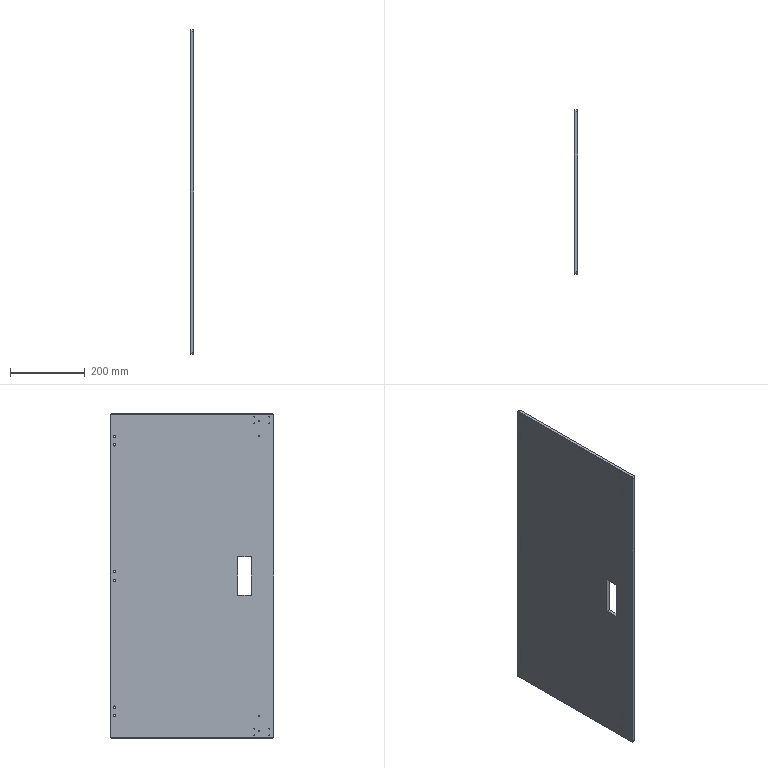Part | NX | 1 solid | 48 faces | box 10 x 438 x 869 mm | volume 3762566 mm3 | cylinder 22 | plane 18 | cone 8 | commonest cylinder face diameters 2.5 x8 6.5 x6 3.3 x4 10 x4
STEP:
#1=CARTESIAN_POINT('',(0.,-398.,-372.204));
#2=VERTEX_POINT('',#1);
#3=CARTESIAN_POINT('',(0.,-398.,-373.854));
#4=DIRECTION('',(-1.,0.,0.));
#5=DIRECTION('',(0.,0.,1.));
#6=AXIS2_PLACEMENT_3D('',#3,#4,#5);
#7=CIRCLE('',#6,1.65);
#8=EDGE_CURVE('',#2,#2,#7,.T.);
#9=ORIENTED_EDGE('',*,*,#8,.F.);
#10=EDGE_LOOP('',(#9));
#11=FACE_BOUND('',#10,.T.);
#12=CARTESIAN_POINT('',(0.,-398.,415.504));
#13=VERTEX_POINT('',#12);
#14=CARTESIAN_POINT('',(0.,-398.,413.854));
#15=DIRECTION('',(-1.,0.,0.));
#16=DIRECTION('',(0.,0.,1.));
#17=AXIS2_PLACEMENT_3D('',#14,#15,#16);
#18=CIRCLE('',#17,1.65);
#19=EDGE_CURVE('',#13,#13,#18,.T.);
#20=ORIENTED_EDGE('',*,*,#19,.F.);
#21=EDGE_LOOP('',(#20));
#22=FACE_BOUND('',#21,.T.);
#23=CARTESIAN_POINT('',(0.,-398.,375.504));
#24=VERTEX_POINT('',#23);
#25=CARTESIAN_POINT('',(0.,-398.,373.854));
#26=DIRECTION('',(-1.,0.,0.));
#27=DIRECTION('',(0.,0.,1.));
#28=AXIS2_PLACEMENT_3D('',#25,#26,#27);
#29=CIRCLE('',#28,1.65);
#30=EDGE_CURVE('',#24,#24,#29,.T.);
#31=ORIENTED_EDGE('',*,*,#30,.F.);
#32=EDGE_LOOP('',(#31));
#33=FACE_BOUND('',#32,.T.);
#34=CARTESIAN_POINT('',(0.,-386.,407.25));
#35=VERTEX_POINT('',#34);
#36=CARTESIAN_POINT('',(0.,-386.,408.5));
#37=DIRECTION('',(1.,0.,0.));
#38=DIRECTION('',(0.,0.,-1.));
#39=AXIS2_PLACEMENT_3D('',#36,#37,#38);
#40=CIRCLE('',#39,1.25);
#41=EDGE_CURVE('',#35,#35,#40,.T.);
#42=ORIENTED_EDGE('',*,*,#41,.T.);
#43=EDGE_LOOP('',(#42));
#44=FACE_BOUND('',#43,.T.);
#45=CARTESIAN_POINT('',(0.,-426.,407.25));
#46=VERTEX_POINT('',#45);
#47=CARTESIAN_POINT('',(0.,-426.,408.5));
#48=DIRECTION('',(1.,0.,0.));
#49=DIRECTION('',(0.,0.,-1.));
#50=AXIS2_PLACEMENT_3D('',#47,#48,#49);
#51=CIRCLE('',#50,1.25);
#52=EDGE_CURVE('',#46,#46,#51,.T.);
#53=ORIENTED_EDGE('',*,*,#52,.T.);
#54=EDGE_LOOP('',(#53));
#55=FACE_BOUND('',#54,.T.);
#56=CARTESIAN_POINT('',(0.,-426.,425.25));
#57=VERTEX_POINT('',#56);
#58=CARTESIAN_POINT('',(0.,-426.,426.5));
#59=DIRECTION('',(1.,0.,0.));
#60=DIRECTION('',(0.,0.,-1.));
#61=AXIS2_PLACEMENT_3D('',#58,#59,#60);
#62=CIRCLE('',#61,1.25);
#63=EDGE_CURVE('',#57,#57,#62,.T.);
#64=ORIENTED_EDGE('',*,*,#63,.T.);
#65=EDGE_LOOP('',(#64));
#66=FACE_BOUND('',#65,.T.);
#67=CARTESIAN_POINT('',(0.,-386.,425.25));
#68=VERTEX_POINT('',#67);
#69=CARTESIAN_POINT('',(0.,-386.,426.5));
#70=DIRECTION('',(1.,0.,0.));
#71=DIRECTION('',(0.,0.,-1.));
#72=AXIS2_PLACEMENT_3D('',#69,#70,#71);
#73=CIRCLE('',#72,1.25);
#74=EDGE_CURVE('',#68,#68,#73,.T.);
#75=ORIENTED_EDGE('',*,*,#74,.T.);
#76=EDGE_LOOP('',(#75));
#77=FACE_BOUND('',#76,.T.);
#78=CARTESIAN_POINT('',(0.,-386.,-427.75));
#79=VERTEX_POINT('',#78);
#80=CARTESIAN_POINT('',(0.,-386.,-426.5));
#81=DIRECTION('',(1.,0.,0.));
#82=DIRECTION('',(0.,0.,-1.));
#83=AXIS2_PLACEMENT_3D('',#80,#81,#82);
#84=CIRCLE('',#83,1.25);
#85=EDGE_CURVE('',#79,#79,#84,.T.);
#86=ORIENTED_EDGE('',*,*,#85,.T.);
#87=EDGE_LOOP('',(#86));
#88=FACE_BOUND('',#87,.T.);
#89=CARTESIAN_POINT('',(0.,-426.,-427.75));
#90=VERTEX_POINT('',#89);
#91=CARTESIAN_POINT('',(0.,-426.,-426.5));
#92=DIRECTION('',(1.,0.,0.));
#93=DIRECTION('',(0.,0.,-1.));
#94=AXIS2_PLACEMENT_3D('',#91,#92,#93);
#95=CIRCLE('',#94,1.25);
#96=EDGE_CURVE('',#90,#90,#95,.T.);
#97=ORIENTED_EDGE('',*,*,#96,.T.);
#98=EDGE_LOOP('',(#97));
#99=FACE_BOUND('',#98,.T.);
#100=CARTESIAN_POINT('',(0.,-426.,-409.75));
#101=VERTEX_POINT('',#100);
#102=CARTESIAN_POINT('',(0.,-426.,-408.5));
#103=DIRECTION('',(1.,0.,0.));
#104=DIRECTION('',(0.,0.,-1.));
#105=AXIS2_PLACEMENT_3D('',#102,#103,#104);
#106=CIRCLE('',#105,1.25);
#107=EDGE_CURVE('',#101,#101,#106,.T.);
#108=ORIENTED_EDGE('',*,*,#107,.T.);
#109=EDGE_LOOP('',(#108));
#110=FACE_BOUND('',#109,.T.);
#111=CARTESIAN_POINT('',(0.,-386.,-409.75));
#112=VERTEX_POINT('',#111);
#113=CARTESIAN_POINT('',(0.,-386.,-408.5));
#114=DIRECTION('',(1.,0.,0.));
#115=DIRECTION('',(0.,0.,-1.));
#116=AXIS2_PLACEMENT_3D('',#113,#114,#115);
#117=CIRCLE('',#116,1.25);
#118=EDGE_CURVE('',#112,#112,#117,.T.);
#119=ORIENTED_EDGE('',*,*,#118,.T.);
#120=EDGE_LOOP('',(#119));
#121=FACE_BOUND('',#120,.T.);
#122=CARTESIAN_POINT('',(0.,-5.,433.5));
#123=VERTEX_POINT('',#122);
#124=CARTESIAN_POINT('',(0.,-1.,429.5));
#125=VERTEX_POINT('',#124);
#126=CARTESIAN_POINT('',(0.,-5.,429.5));
#127=DIRECTION('',(1.,0.,0.));
#128=DIRECTION('',(0.,0.,-1.));
#129=AXIS2_PLACEMENT_3D('',#126,#127,#128);
#130=CIRCLE('',#129,4.);
#131=EDGE_CURVE('',#123,#125,#130,.F.);
#132=ORIENTED_EDGE('',*,*,#131,.T.);
#133=CARTESIAN_POINT('',(0.,-1.,-429.5));
#134=VERTEX_POINT('',#133);
#135=CARTESIAN_POINT('',(0.,-1.,434.5));
#136=DIRECTION('',(0.,0.,-1.));
#137=VECTOR('',#136,1000.);
#138=LINE('',#135,#137);
#139=EDGE_CURVE('',#125,#134,#138,.T.);
#140=ORIENTED_EDGE('',*,*,#139,.T.);
#141=CARTESIAN_POINT('',(0.,-5.,-433.5));
#142=VERTEX_POINT('',#141);
#143=CARTESIAN_POINT('',(0.,-5.,-429.5));
#144=DIRECTION('',(1.,0.,0.));
#145=DIRECTION('',(0.,0.,-1.));
#146=AXIS2_PLACEMENT_3D('',#143,#144,#145);
#147=CIRCLE('',#146,4.);
#148=EDGE_CURVE('',#134,#142,#147,.F.);
#149=ORIENTED_EDGE('',*,*,#148,.T.);
#150=CARTESIAN_POINT('',(0.,-433.,-433.5));
#151=VERTEX_POINT('',#150);
#152=CARTESIAN_POINT('',(0.,-433.,-433.5));
#153=DIRECTION('',(0.,-1.,0.));
#154=VECTOR('',#153,1000.);
#155=LINE('',#152,#154);
#156=EDGE_CURVE('',#142,#151,#155,.T.);
#157=ORIENTED_EDGE('',*,*,#156,.T.);
#158=CARTESIAN_POINT('',(0.,-437.,-429.5));
#159=VERTEX_POINT('',#158);
#160=CARTESIAN_POINT('',(0.,-433.,-429.5));
#161=DIRECTION('',(1.,0.,0.));
#162=DIRECTION('',(0.,0.,-1.));
#163=AXIS2_PLACEMENT_3D('',#160,#161,#162);
#164=CIRCLE('',#163,4.);
#165=EDGE_CURVE('',#151,#159,#164,.F.);
#166=ORIENTED_EDGE('',*,*,#165,.T.);
#167=CARTESIAN_POINT('',(0.,-437.,429.5));
#168=VERTEX_POINT('',#167);
#169=CARTESIAN_POINT('',(0.,-437.,434.5));
#170=DIRECTION('',(0.,0.,1.));
#171=VECTOR('',#170,1000.);
#172=LINE('',#169,#171);
#173=EDGE_CURVE('',#159,#168,#172,.T.);
#174=ORIENTED_EDGE('',*,*,#173,.T.);
#175=CARTESIAN_POINT('',(0.,-433.,433.5));
#176=VERTEX_POINT('',#175);
#177=CARTESIAN_POINT('',(0.,-433.,429.5));
#178=DIRECTION('',(1.,0.,0.));
#179=DIRECTION('',(0.,0.,-1.));
#180=AXIS2_PLACEMENT_3D('',#177,#178,#179);
#181=CIRCLE('',#180,4.);
#182=EDGE_CURVE('',#168,#176,#181,.F.);
#183=ORIENTED_EDGE('',*,*,#182,.T.);
#184=CARTESIAN_POINT('',(0.,-438.,433.5));
#185=DIRECTION('',(0.,1.,0.));
#186=VECTOR('',#185,1000.);
#187=LINE('',#184,#186);
#188=EDGE_CURVE('',#176,#123,#187,.T.);
#189=ORIENTED_EDGE('',*,*,#188,.T.);
#190=EDGE_LOOP('',(#132,#140,#149,#157,#166,#174,#183,#189));
#191=FACE_BOUND('',#190,.T.);
#192=CARTESIAN_POINT('',(0.,-12.,-377.25));
#193=VERTEX_POINT('',#192);
#194=CARTESIAN_POINT('',(0.,-12.,-374.));
#195=DIRECTION('',(1.,0.,0.));
#196=DIRECTION('',(0.,0.,-1.));
#197=AXIS2_PLACEMENT_3D('',#194,#195,#196);
#198=CIRCLE('',#197,3.25);
#199=EDGE_CURVE('',#193,#193,#198,.T.);
#200=ORIENTED_EDGE('',*,*,#199,.T.);
#201=EDGE_LOOP('',(#200));
#202=FACE_BOUND('',#201,.T.);
#203=CARTESIAN_POINT('',(0.,-12.,-354.25));
#204=VERTEX_POINT('',#203);
#205=CARTESIAN_POINT('',(0.,-12.,-351.));
#206=DIRECTION('',(1.,0.,0.));
#207=DIRECTION('',(0.,0.,-1.));
#208=AXIS2_PLACEMENT_3D('',#205,#206,#207);
#209=CIRCLE('',#208,3.25);
#210=EDGE_CURVE('',#204,#204,#209,.T.);
#211=ORIENTED_EDGE('',*,*,#210,.T.);
#212=EDGE_LOOP('',(#211));
#213=FACE_BOUND('',#212,.T.);
#214=CARTESIAN_POINT('',(0.,-12.,347.75));
#215=VERTEX_POINT('',#214);
#216=CARTESIAN_POINT('',(0.,-12.,351.));
#217=DIRECTION('',(1.,0.,0.));
#218=DIRECTION('',(0.,0.,-1.));
#219=AXIS2_PLACEMENT_3D('',#216,#217,#218);
#220=CIRCLE('',#219,3.25);
#221=EDGE_CURVE('',#215,#215,#220,.T.);
#222=ORIENTED_EDGE('',*,*,#221,.T.);
#223=EDGE_LOOP('',(#222));
#224=FACE_BOUND('',#223,.T.);
#225=CARTESIAN_POINT('',(0.,-12.,370.75));
#226=VERTEX_POINT('',#225);
#227=CARTESIAN_POINT('',(0.,-12.,374.));
#228=DIRECTION('',(1.,0.,0.));
#229=DIRECTION('',(0.,0.,-1.));
#230=AXIS2_PLACEMENT_3D('',#227,#228,#229);
#231=CIRCLE('',#230,3.25);
#232=EDGE_CURVE('',#226,#226,#231,.T.);
#233=ORIENTED_EDGE('',*,*,#232,.T.);
#234=EDGE_LOOP('',(#233));
#235=FACE_BOUND('',#234,.T.);
#236=CARTESIAN_POINT('',(0.,-12.,8.25));
#237=VERTEX_POINT('',#236);
#238=CARTESIAN_POINT('',(0.,-12.,11.5));
#239=DIRECTION('',(1.,0.,0.));
#240=DIRECTION('',(0.,0.,-1.));
#241=AXIS2_PLACEMENT_3D('',#238,#239,#240);
#242=CIRCLE('',#241,3.25);
#243=EDGE_CURVE('',#237,#237,#242,.T.);
#244=ORIENTED_EDGE('',*,*,#243,.T.);
#245=EDGE_LOOP('',(#244));
#246=FACE_BOUND('',#245,.T.);
#247=CARTESIAN_POINT('',(0.,-12.,-14.75));
#248=VERTEX_POINT('',#247);
#249=CARTESIAN_POINT('',(0.,-12.,-11.5));
#250=DIRECTION('',(1.,0.,0.));
#251=DIRECTION('',(0.,0.,-1.));
#252=AXIS2_PLACEMENT_3D('',#249,#250,#251);
#253=CIRCLE('',#252,3.25);
#254=EDGE_CURVE('',#248,#248,#253,.T.);
#255=ORIENTED_EDGE('',*,*,#254,.T.);
#256=EDGE_LOOP('',(#255));
#257=FACE_BOUND('',#256,.T.);
#258=CARTESIAN_POINT('',(0.,-378.,51.5));
#259=VERTEX_POINT('',#258);
#260=CARTESIAN_POINT('',(0.,-378.,-51.5));
#261=VERTEX_POINT('',#260);
#262=CARTESIAN_POINT('',(0.,-378.,51.5));
#263=DIRECTION('',(0.,0.,-1.));
#264=VECTOR('',#263,1000.);
#265=LINE('',#262,#264);
#266=EDGE_CURVE('',#259,#261,#265,.T.);
#267=ORIENTED_EDGE('',*,*,#266,.T.);
#268=CARTESIAN_POINT('',(0.,-341.,-51.5));
#269=VERTEX_POINT('',#268);
#270=CARTESIAN_POINT('',(0.,-341.,-51.5));
#271=DIRECTION('',(0.,1.,0.));
#272=VECTOR('',#271,1000.);
#273=LINE('',#270,#272);
#274=EDGE_CURVE('',#261,#269,#273,.T.);
#275=ORIENTED_EDGE('',*,*,#274,.T.);
#276=CARTESIAN_POINT('',(0.,-341.,51.5));
#277=VERTEX_POINT('',#276);
#278=CARTESIAN_POINT('',(0.,-341.,51.5));
#279=DIRECTION('',(0.,0.,1.));
#280=VECTOR('',#279,1000.);
#281=LINE('',#278,#280);
#282=EDGE_CURVE('',#269,#277,#281,.T.);
#283=ORIENTED_EDGE('',*,*,#282,.T.);
#284=CARTESIAN_POINT('',(0.,-341.,51.5));
#285=DIRECTION('',(0.,-1.,0.));
#286=VECTOR('',#285,1000.);
#287=LINE('',#284,#286);
#288=EDGE_CURVE('',#277,#259,#287,.T.);
#289=ORIENTED_EDGE('',*,*,#288,.T.);
#290=EDGE_LOOP('',(#267,#275,#283,#289));
#291=FACE_BOUND('',#290,.T.);
#292=CARTESIAN_POINT('',(0.,-398.,-412.204));
#293=VERTEX_POINT('',#292);
#294=CARTESIAN_POINT('',(0.,-398.,-413.854));
#295=DIRECTION('',(-1.,0.,0.));
#296=DIRECTION('',(0.,0.,1.));
#297=AXIS2_PLACEMENT_3D('',#294,#295,#296);
#298=CIRCLE('',#297,1.65);
#299=EDGE_CURVE('',#293,#293,#298,.T.);
#300=ORIENTED_EDGE('',*,*,#299,.F.);
#301=EDGE_LOOP('',(#300));
#302=FACE_BOUND('',#301,.T.);
#303=CARTESIAN_POINT('',(0.,-438.,434.5));
#304=DIRECTION('',(1.,0.,0.));
#305=DIRECTION('',(0.,0.,-1.));
#306=AXIS2_PLACEMENT_3D('',#303,#304,#305);
#307=PLANE('',#306);
#308=ADVANCED_FACE('',(#11,#22,#33,#44,#55,#66,#77,#88,#99,#110,#121,#191,#202,#213,#224,#235,#246,#257,#291,#302),#307,.F.);
#309=CARTESIAN_POINT('',(1.,-438.,-429.5));
#310=VERTEX_POINT('',#309);
#311=CARTESIAN_POINT('',(9.,-438.,-429.5));
#312=VERTEX_POINT('',#311);
#313=CARTESIAN_POINT('',(10.,-438.,-429.5));
#314=DIRECTION('',(1.,0.,0.));
#315=VECTOR('',#314,1000.);
#316=LINE('',#313,#315);
#317=EDGE_CURVE('',#310,#312,#316,.T.);
#318=ORIENTED_EDGE('',*,*,#317,.T.);
#319=CARTESIAN_POINT('',(9.,-438.,429.5));
#320=VERTEX_POINT('',#319);
#321=CARTESIAN_POINT('',(9.,-438.,434.5));
#322=DIRECTION('',(0.,0.,1.));
#323=VECTOR('',#322,1000.);
#324=LINE('',#321,#323);
#325=EDGE_CURVE('',#312,#320,#324,.T.);
#326=ORIENTED_EDGE('',*,*,#325,.T.);
#327=CARTESIAN_POINT('',(1.,-438.,429.5));
#328=VERTEX_POINT('',#327);
#329=CARTESIAN_POINT('',(10.,-438.,429.5));
#330=DIRECTION('',(1.,0.,0.));
#331=VECTOR('',#330,1000.);
#332=LINE('',#329,#331);
#333=EDGE_CURVE('',#320,#328,#332,.F.);
#334=ORIENTED_EDGE('',*,*,#333,.T.);
#335=CARTESIAN_POINT('',(1.,-438.,434.5));
#336=DIRECTION('',(0.,0.,-1.));
#337=VECTOR('',#336,1000.);
#338=LINE('',#335,#337);
#339=EDGE_CURVE('',#328,#310,#338,.T.);
#340=ORIENTED_EDGE('',*,*,#339,.T.);
#341=EDGE_LOOP('',(#318,#326,#334,#340));
#342=FACE_BOUND('',#341,.T.);
#343=CARTESIAN_POINT('',(10.,-438.,434.5));
#344=DIRECTION('',(0.,1.,0.));
#345=DIRECTION('',(0.,0.,1.));
#346=AXIS2_PLACEMENT_3D('',#343,#344,#345);
#347=PLANE('',#346);
#348=ADVANCED_FACE('',(#342),#347,.F.);
#349=CARTESIAN_POINT('',(10.,-398.,-412.204));
#350=VERTEX_POINT('',#349);
#351=CARTESIAN_POINT('',(10.,-398.,-413.854));
#352=DIRECTION('',(-1.,0.,0.));
#353=DIRECTION('',(0.,0.,1.));
#354=AXIS2_PLACEMENT_3D('',#351,#352,#353);
#355=CIRCLE('',#354,1.65);
#356=EDGE_CURVE('',#350,#350,#355,.T.);
#357=ORIENTED_EDGE('',*,*,#356,.T.);
#358=EDGE_LOOP('',(#357));
#359=FACE_BOUND('',#358,.T.);
#360=CARTESIAN_POINT('',(10.,-398.,-372.204));
#361=VERTEX_POINT('',#360);
#362=CARTESIAN_POINT('',(10.,-398.,-373.854));
#363=DIRECTION('',(-1.,0.,0.));
#364=DIRECTION('',(0.,0.,1.));
#365=AXIS2_PLACEMENT_3D('',#362,#363,#364);
#366=CIRCLE('',#365,1.65);
#367=EDGE_CURVE('',#361,#361,#366,.T.);
#368=ORIENTED_EDGE('',*,*,#367,.T.);
#369=EDGE_LOOP('',(#368));
#370=FACE_BOUND('',#369,.T.);
#371=CARTESIAN_POINT('',(10.,-398.,415.504));
#372=VERTEX_POINT('',#371);
#373=CARTESIAN_POINT('',(10.,-398.,413.854));
#374=DIRECTION('',(-1.,0.,0.));
#375=DIRECTION('',(0.,0.,1.));
#376=AXIS2_PLACEMENT_3D('',#373,#374,#375);
#377=CIRCLE('',#376,1.65);
#378=EDGE_CURVE('',#372,#372,#377,.T.);
#379=ORIENTED_EDGE('',*,*,#378,.T.);
#380=EDGE_LOOP('',(#379));
#381=FACE_BOUND('',#380,.T.);
#382=CARTESIAN_POINT('',(10.,-398.,375.504));
#383=VERTEX_POINT('',#382);
#384=CARTESIAN_POINT('',(10.,-398.,373.854));
#385=DIRECTION('',(-1.,0.,0.));
#386=DIRECTION('',(0.,0.,1.));
#387=AXIS2_PLACEMENT_3D('',#384,#385,#386);
#388=CIRCLE('',#387,1.65);
#389=EDGE_CURVE('',#383,#383,#388,.T.);
#390=ORIENTED_EDGE('',*,*,#389,.T.);
#391=EDGE_LOOP('',(#390));
#392=FACE_BOUND('',#391,.T.);
#393=CARTESIAN_POINT('',(10.,-386.,407.25));
#394=VERTEX_POINT('',#393);
#395=CARTESIAN_POINT('',(10.,-386.,408.5));
#396=DIRECTION('',(1.,0.,0.));
#397=DIRECTION('',(0.,0.,-1.));
#398=AXIS2_PLACEMENT_3D('',#395,#396,#397);
#399=CIRCLE('',#398,1.25);
#400=EDGE_CURVE('',#394,#394,#399,.T.);
#401=ORIENTED_EDGE('',*,*,#400,.F.);
#402=EDGE_LOOP('',(#401));
#403=FACE_BOUND('',#402,.T.);
#404=CARTESIAN_POINT('',(10.,-426.,407.25));
#405=VERTEX_POINT('',#404);
#406=CARTESIAN_POINT('',(10.,-426.,408.5));
#407=DIRECTION('',(1.,0.,0.));
#408=DIRECTION('',(0.,0.,-1.));
#409=AXIS2_PLACEMENT_3D('',#406,#407,#408);
#410=CIRCLE('',#409,1.25);
#411=EDGE_CURVE('',#405,#405,#410,.T.);
#412=ORIENTED_EDGE('',*,*,#411,.F.);
#413=EDGE_LOOP('',(#412));
#414=FACE_BOUND('',#413,.T.);
#415=CARTESIAN_POINT('',(10.,-426.,425.25));
#416=VERTEX_POINT('',#415);
#417=CARTESIAN_POINT('',(10.,-426.,426.5));
#418=DIRECTION('',(1.,0.,0.));
#419=DIRECTION('',(0.,0.,-1.));
#420=AXIS2_PLACEMENT_3D('',#417,#418,#419);
#421=CIRCLE('',#420,1.25);
#422=EDGE_CURVE('',#416,#416,#421,.T.);
#423=ORIENTED_EDGE('',*,*,#422,.F.);
#424=EDGE_LOOP('',(#423));
#425=FACE_BOUND('',#424,.T.);
#426=CARTESIAN_POINT('',(10.,-386.,425.25));
#427=VERTEX_POINT('',#426);
#428=CARTESIAN_POINT('',(10.,-386.,426.5));
#429=DIRECTION('',(1.,0.,0.));
#430=DIRECTION('',(0.,0.,-1.));
#431=AXIS2_PLACEMENT_3D('',#428,#429,#430);
#432=CIRCLE('',#431,1.25);
#433=EDGE_CURVE('',#427,#427,#432,.T.);
#434=ORIENTED_EDGE('',*,*,#433,.F.);
#435=EDGE_LOOP('',(#434));
#436=FACE_BOUND('',#435,.T.);
#437=CARTESIAN_POINT('',(10.,-386.,-427.75));
#438=VERTEX_POINT('',#437);
#439=CARTESIAN_POINT('',(10.,-386.,-426.5));
#440=DIRECTION('',(1.,0.,0.));
#441=DIRECTION('',(0.,0.,-1.));
#442=AXIS2_PLACEMENT_3D('',#439,#440,#441);
#443=CIRCLE('',#442,1.25);
#444=EDGE_CURVE('',#438,#438,#443,.T.);
#445=ORIENTED_EDGE('',*,*,#444,.F.);
#446=EDGE_LOOP('',(#445));
#447=FACE_BOUND('',#446,.T.);
#448=CARTESIAN_POINT('',(10.,-426.,-427.75));
#449=VERTEX_POINT('',#448);
#450=CARTESIAN_POINT('',(10.,-426.,-426.5));
#451=DIRECTION('',(1.,0.,0.));
#452=DIRECTION('',(0.,0.,-1.));
#453=AXIS2_PLACEMENT_3D('',#450,#451,#452);
#454=CIRCLE('',#453,1.25);
#455=EDGE_CURVE('',#449,#449,#454,.T.);
#456=ORIENTED_EDGE('',*,*,#455,.F.);
#457=EDGE_LOOP('',(#456));
#458=FACE_BOUND('',#457,.T.);
#459=CARTESIAN_POINT('',(10.,-426.,-409.75));
#460=VERTEX_POINT('',#459);
#461=CARTESIAN_POINT('',(10.,-426.,-408.5));
#462=DIRECTION('',(1.,0.,0.));
#463=DIRECTION('',(0.,0.,-1.));
#464=AXIS2_PLACEMENT_3D('',#461,#462,#463);
#465=CIRCLE('',#464,1.25);
#466=EDGE_CURVE('',#460,#460,#465,.T.);
#467=ORIENTED_EDGE('',*,*,#466,.F.);
#468=EDGE_LOOP('',(#467));
#469=FACE_BOUND('',#468,.T.);
#470=CARTESIAN_POINT('',(10.,-386.,-409.75));
#471=VERTEX_POINT('',#470);
#472=CARTESIAN_POINT('',(10.,-386.,-408.5));
#473=DIRECTION('',(1.,0.,0.));
#474=DIRECTION('',(0.,0.,-1.));
#475=AXIS2_PLACEMENT_3D('',#472,#473,#474);
#476=CIRCLE('',#475,1.25);
#477=EDGE_CURVE('',#471,#471,#476,.T.);
#478=ORIENTED_EDGE('',*,*,#477,.F.);
#479=EDGE_LOOP('',(#478));
#480=FACE_BOUND('',#479,.T.);
#481=CARTESIAN_POINT('',(10.,-5.,-433.5));
#482=VERTEX_POINT('',#481);
#483=CARTESIAN_POINT('',(10.,-1.,-429.5));
#484=VERTEX_POINT('',#483);
#485=CARTESIAN_POINT('',(10.,-5.,-429.5));
#486=DIRECTION('',(-1.,0.,0.));
#487=DIRECTION('',(0.,-1.,0.));
#488=AXIS2_PLACEMENT_3D('',#485,#486,#487);
#489=CIRCLE('',#488,4.);
#490=EDGE_CURVE('',#482,#484,#489,.F.);
#491=ORIENTED_EDGE('',*,*,#490,.T.);
#492=CARTESIAN_POINT('',(10.,-1.,429.5));
#493=VERTEX_POINT('',#492);
#494=CARTESIAN_POINT('',(10.,-1.,434.5));
#495=DIRECTION('',(0.,0.,1.));
#496=VECTOR('',#495,1000.);
#497=LINE('',#494,#496);
#498=EDGE_CURVE('',#484,#493,#497,.T.);
#499=ORIENTED_EDGE('',*,*,#498,.T.);
#500=CARTESIAN_POINT('',(10.,-5.,433.5));
#501=VERTEX_POINT('',#500);
#502=CARTESIAN_POINT('',(10.,-5.,429.5));
#503=DIRECTION('',(-1.,0.,0.));
#504=DIRECTION('',(0.,-1.,0.));
#505=AXIS2_PLACEMENT_3D('',#502,#503,#504);
#506=CIRCLE('',#505,4.);
#507=EDGE_CURVE('',#493,#501,#506,.F.);
#508=ORIENTED_EDGE('',*,*,#507,.T.);
#509=CARTESIAN_POINT('',(10.,-433.,433.5));
#510=VERTEX_POINT('',#509);
#511=CARTESIAN_POINT('',(10.,0.,433.5));
#512=DIRECTION('',(0.,-1.,0.));
#513=VECTOR('',#512,1000.);
#514=LINE('',#511,#513);
#515=EDGE_CURVE('',#501,#510,#514,.T.);
#516=ORIENTED_EDGE('',*,*,#515,.T.);
#517=CARTESIAN_POINT('',(10.,-437.,429.5));
#518=VERTEX_POINT('',#517);
#519=CARTESIAN_POINT('',(10.,-433.,429.5));
#520=DIRECTION('',(-1.,0.,0.));
#521=DIRECTION('',(0.,-1.,0.));
#522=AXIS2_PLACEMENT_3D('',#519,#520,#521);
#523=CIRCLE('',#522,4.);
#524=EDGE_CURVE('',#510,#518,#523,.F.);
#525=ORIENTED_EDGE('',*,*,#524,.T.);
#526=CARTESIAN_POINT('',(10.,-437.,-429.5));
#527=VERTEX_POINT('',#526);
#528=CARTESIAN_POINT('',(10.,-437.,434.5));
#529=DIRECTION('',(0.,0.,-1.));
#530=VECTOR('',#529,1000.);
#531=LINE('',#528,#530);
#532=EDGE_CURVE('',#518,#527,#531,.T.);
#533=ORIENTED_EDGE('',*,*,#532,.T.);
#534=CARTESIAN_POINT('',(10.,-433.,-433.5));
#535=VERTEX_POINT('',#534);
#536=CARTESIAN_POINT('',(10.,-433.,-429.5));
#537=DIRECTION('',(-1.,0.,0.));
#538=DIRECTION('',(0.,-1.,0.));
#539=AXIS2_PLACEMENT_3D('',#536,#537,#538);
#540=CIRCLE('',#539,4.);
#541=EDGE_CURVE('',#527,#535,#540,.F.);
#542=ORIENTED_EDGE('',*,*,#541,.T.);
#543=CARTESIAN_POINT('',(10.,-5.,-433.5));
#544=DIRECTION('',(0.,1.,0.));
#545=VECTOR('',#544,1000.);
#546=LINE('',#543,#545);
#547=EDGE_CURVE('',#535,#482,#546,.T.);
#548=ORIENTED_EDGE('',*,*,#547,.T.);
#549=EDGE_LOOP('',(#491,#499,#508,#516,#525,#533,#542,#548));
#550=FACE_BOUND('',#549,.T.);
#551=CARTESIAN_POINT('',(10.,-12.,-377.25));
#552=VERTEX_POINT('',#551);
#553=CARTESIAN_POINT('',(10.,-12.,-374.));
#554=DIRECTION('',(1.,0.,0.));
#555=DIRECTION('',(0.,0.,-1.));
#556=AXIS2_PLACEMENT_3D('',#553,#554,#555);
#557=CIRCLE('',#556,3.25);
#558=EDGE_CURVE('',#552,#552,#557,.T.);
#559=ORIENTED_EDGE('',*,*,#558,.F.);
#560=EDGE_LOOP('',(#559));
#561=FACE_BOUND('',#560,.T.);
#562=CARTESIAN_POINT('',(10.,-12.,-354.25));
#563=VERTEX_POINT('',#562);
#564=CARTESIAN_POINT('',(10.,-12.,-351.));
#565=DIRECTION('',(1.,0.,0.));
#566=DIRECTION('',(0.,0.,-1.));
#567=AXIS2_PLACEMENT_3D('',#564,#565,#566);
#568=CIRCLE('',#567,3.25);
#569=EDGE_CURVE('',#563,#563,#568,.T.);
#570=ORIENTED_EDGE('',*,*,#569,.F.);
#571=EDGE_LOOP('',(#570));
#572=FACE_BOUND('',#571,.T.);
#573=CARTESIAN_POINT('',(10.,-12.,347.75));
#574=VERTEX_POINT('',#573);
#575=CARTESIAN_POINT('',(10.,-12.,351.));
#576=DIRECTION('',(1.,0.,0.));
#577=DIRECTION('',(0.,0.,-1.));
#578=AXIS2_PLACEMENT_3D('',#575,#576,#577);
#579=CIRCLE('',#578,3.25);
#580=EDGE_CURVE('',#574,#574,#579,.T.);
#581=ORIENTED_EDGE('',*,*,#580,.F.);
#582=EDGE_LOOP('',(#581));
#583=FACE_BOUND('',#582,.T.);
#584=CARTESIAN_POINT('',(10.,-12.,370.75));
#585=VERTEX_POINT('',#584);
#586=CARTESIAN_POINT('',(10.,-12.,374.));
#587=DIRECTION('',(1.,0.,0.));
#588=DIRECTION('',(0.,0.,-1.));
#589=AXIS2_PLACEMENT_3D('',#586,#587,#588);
#590=CIRCLE('',#589,3.25);
#591=EDGE_CURVE('',#585,#585,#590,.T.);
#592=ORIENTED_EDGE('',*,*,#591,.F.);
#593=EDGE_LOOP('',(#592));
#594=FACE_BOUND('',#593,.T.);
#595=CARTESIAN_POINT('',(10.,-12.,8.25));
#596=VERTEX_POINT('',#595);
#597=CARTESIAN_POINT('',(10.,-12.,11.5));
#598=DIRECTION('',(1.,0.,0.));
#599=DIRECTION('',(0.,0.,-1.));
#600=AXIS2_PLACEMENT_3D('',#597,#598,#599);
#601=CIRCLE('',#600,3.25);
#602=EDGE_CURVE('',#596,#596,#601,.T.);
#603=ORIENTED_EDGE('',*,*,#602,.F.);
#604=EDGE_LOOP('',(#603));
#605=FACE_BOUND('',#604,.T.);
#606=CARTESIAN_POINT('',(10.,-12.,-14.75));
#607=VERTEX_POINT('',#606);
#608=CARTESIAN_POINT('',(10.,-12.,-11.5));
#609=DIRECTION('',(1.,0.,0.));
#610=DIRECTION('',(0.,0.,-1.));
#611=AXIS2_PLACEMENT_3D('',#608,#609,#610);
#612=CIRCLE('',#611,3.25);
#613=EDGE_CURVE('',#607,#607,#612,.T.);
#614=ORIENTED_EDGE('',*,*,#613,.F.);
#615=EDGE_LOOP('',(#614));
#616=FACE_BOUND('',#615,.T.);
#617=CARTESIAN_POINT('',(10.,-341.,-51.5));
#618=VERTEX_POINT('',#617);
#619=CARTESIAN_POINT('',(10.,-341.,51.5));
#620=VERTEX_POINT('',#619);
#621=CARTESIAN_POINT('',(10.,-341.,51.5));
#622=DIRECTION('',(0.,0.,1.));
#623=VECTOR('',#622,1000.);
#624=LINE('',#621,#623);
#625=EDGE_CURVE('',#618,#620,#624,.T.);
#626=ORIENTED_EDGE('',*,*,#625,.F.);
#627=CARTESIAN_POINT('',(10.,-378.,-51.5));
#628=VERTEX_POINT('',#627);
#629=CARTESIAN_POINT('',(10.,-341.,-51.5));
#630=DIRECTION('',(0.,1.,0.));
#631=VECTOR('',#630,1000.);
#632=LINE('',#629,#631);
#633=EDGE_CURVE('',#628,#618,#632,.T.);
#634=ORIENTED_EDGE('',*,*,#633,.F.);
#635=CARTESIAN_POINT('',(10.,-378.,51.5));
#636=VERTEX_POINT('',#635);
#637=CARTESIAN_POINT('',(10.,-378.,51.5));
#638=DIRECTION('',(0.,0.,-1.));
#639=VECTOR('',#638,1000.);
#640=LINE('',#637,#639);
#641=EDGE_CURVE('',#636,#628,#640,.T.);
#642=ORIENTED_EDGE('',*,*,#641,.F.);
#643=CARTESIAN_POINT('',(10.,-341.,51.5));
#644=DIRECTION('',(0.,-1.,0.));
#645=VECTOR('',#644,1000.);
#646=LINE('',#643,#645);
#647=EDGE_CURVE('',#620,#636,#646,.T.);
#648=ORIENTED_EDGE('',*,*,#647,.F.);
#649=EDGE_LOOP('',(#626,#634,#642,#648));
#650=FACE_BOUND('',#649,.T.);
#651=CARTESIAN_POINT('',(10.,0.,434.5));
#652=DIRECTION('',(-1.,0.,0.));
#653=DIRECTION('',(0.,-1.,0.));
#654=AXIS2_PLACEMENT_3D('',#651,#652,#653);
#655=PLANE('',#654);
#656=ADVANCED_FACE('',(#359,#370,#381,#392,#403,#414,#425,#436,#447,#458,#469,#480,#550,#561,#572,#583,#594,#605,#616,#650),#655,.F.);
#657=CARTESIAN_POINT('',(1.,0.,429.5));
#658=VERTEX_POINT('',#657);
#659=CARTESIAN_POINT('',(9.,0.,429.5));
#660=VERTEX_POINT('',#659);
#661=CARTESIAN_POINT('',(0.,0.,429.5));
#662=DIRECTION('',(-1.,0.,0.));
#663=VECTOR('',#662,1000.);
#664=LINE('',#661,#663);
#665=EDGE_CURVE('',#658,#660,#664,.F.);
#666=ORIENTED_EDGE('',*,*,#665,.T.);
#667=CARTESIAN_POINT('',(9.,0.,-429.5));
#668=VERTEX_POINT('',#667);
#669=CARTESIAN_POINT('',(9.,0.,434.5));
#670=DIRECTION('',(0.,0.,-1.));
#671=VECTOR('',#670,1000.);
#672=LINE('',#669,#671);
#673=EDGE_CURVE('',#660,#668,#672,.T.);
#674=ORIENTED_EDGE('',*,*,#673,.T.);
#675=CARTESIAN_POINT('',(1.,0.,-429.5));
#676=VERTEX_POINT('',#675);
#677=CARTESIAN_POINT('',(0.,0.,-429.5));
#678=DIRECTION('',(-1.,0.,0.));
#679=VECTOR('',#678,1000.);
#680=LINE('',#677,#679);
#681=EDGE_CURVE('',#668,#676,#680,.T.);
#682=ORIENTED_EDGE('',*,*,#681,.T.);
#683=CARTESIAN_POINT('',(1.,0.,434.5));
#684=DIRECTION('',(0.,0.,1.));
#685=VECTOR('',#684,1000.);
#686=LINE('',#683,#685);
#687=EDGE_CURVE('',#676,#658,#686,.T.);
#688=ORIENTED_EDGE('',*,*,#687,.T.);
#689=EDGE_LOOP('',(#666,#674,#682,#688));
#690=FACE_BOUND('',#689,.T.);
#691=CARTESIAN_POINT('',(0.,0.,434.5));
#692=DIRECTION('',(0.,-1.,0.));
#693=DIRECTION('',(1.,0.,0.));
#694=AXIS2_PLACEMENT_3D('',#691,#692,#693);
#695=PLANE('',#694);
#696=ADVANCED_FACE('',(#690),#695,.F.);
#697=CARTESIAN_POINT('',(1.,-433.,434.5));
#698=VERTEX_POINT('',#697);
#699=CARTESIAN_POINT('',(9.,-433.,434.5));
#700=VERTEX_POINT('',#699);
#701=CARTESIAN_POINT('',(0.,-433.,434.5));
#702=DIRECTION('',(1.,0.,0.));
#703=VECTOR('',#702,1000.);
#704=LINE('',#701,#703);
#705=EDGE_CURVE('',#698,#700,#704,.T.);
#706=ORIENTED_EDGE('',*,*,#705,.T.);
#707=CARTESIAN_POINT('',(9.,-5.,434.5));
#708=VERTEX_POINT('',#707);
#709=CARTESIAN_POINT('',(9.,0.,434.5));
#710=DIRECTION('',(0.,1.,0.));
#711=VECTOR('',#710,1000.);
#712=LINE('',#709,#711);
#713=EDGE_CURVE('',#700,#708,#712,.T.);
#714=ORIENTED_EDGE('',*,*,#713,.T.);
#715=CARTESIAN_POINT('',(1.,-5.,434.5));
#716=VERTEX_POINT('',#715);
#717=CARTESIAN_POINT('',(0.,-5.,434.5));
#718=DIRECTION('',(-1.,0.,0.));
#719=VECTOR('',#718,1000.);
#720=LINE('',#717,#719);
#721=EDGE_CURVE('',#708,#716,#720,.T.);
#722=ORIENTED_EDGE('',*,*,#721,.T.);
#723=CARTESIAN_POINT('',(1.,0.,434.5));
#724=DIRECTION('',(0.,-1.,0.));
#725=VECTOR('',#724,1000.);
#726=LINE('',#723,#725);
#727=EDGE_CURVE('',#716,#698,#726,.T.);
#728=ORIENTED_EDGE('',*,*,#727,.T.);
#729=EDGE_LOOP('',(#706,#714,#722,#728));
#730=FACE_BOUND('',#729,.T.);
#731=CARTESIAN_POINT('',(0.,0.,434.5));
#732=DIRECTION('',(0.,0.,-1.));
#733=DIRECTION('',(-1.,0.,0.));
#734=AXIS2_PLACEMENT_3D('',#731,#732,#733);
#735=PLANE('',#734);
#736=ADVANCED_FACE('',(#730),#735,.F.);
#737=CARTESIAN_POINT('',(1.,-5.,-434.5));
#738=VERTEX_POINT('',#737);
#739=CARTESIAN_POINT('',(9.,-5.,-434.5));
#740=VERTEX_POINT('',#739);
#741=CARTESIAN_POINT('',(10.,-5.,-434.5));
#742=DIRECTION('',(-1.,0.,0.));
#743=VECTOR('',#742,1000.);
#744=LINE('',#741,#743);
#745=EDGE_CURVE('',#738,#740,#744,.F.);
#746=ORIENTED_EDGE('',*,*,#745,.T.);
#747=CARTESIAN_POINT('',(9.,-433.,-434.5));
#748=VERTEX_POINT('',#747);
#749=CARTESIAN_POINT('',(9.,-433.,-434.5));
#750=DIRECTION('',(0.,-1.,0.));
#751=VECTOR('',#750,1000.);
#752=LINE('',#749,#751);
#753=EDGE_CURVE('',#740,#748,#752,.T.);
#754=ORIENTED_EDGE('',*,*,#753,.T.);
#755=CARTESIAN_POINT('',(1.,-433.,-434.5));
#756=VERTEX_POINT('',#755);
#757=CARTESIAN_POINT('',(0.,-433.,-434.5));
#758=DIRECTION('',(1.,0.,0.));
#759=VECTOR('',#758,1000.);
#760=LINE('',#757,#759);
#761=EDGE_CURVE('',#748,#756,#760,.F.);
#762=ORIENTED_EDGE('',*,*,#761,.T.);
#763=CARTESIAN_POINT('',(1.,-5.,-434.5));
#764=DIRECTION('',(0.,1.,0.));
#765=VECTOR('',#764,1000.);
#766=LINE('',#763,#765);
#767=EDGE_CURVE('',#756,#738,#766,.T.);
#768=ORIENTED_EDGE('',*,*,#767,.T.);
#769=EDGE_LOOP('',(#746,#754,#762,#768));
#770=FACE_BOUND('',#769,.T.);
#771=CARTESIAN_POINT('',(0.,0.,-434.5));
#772=DIRECTION('',(0.,0.,-1.));
#773=DIRECTION('',(-1.,0.,0.));
#774=AXIS2_PLACEMENT_3D('',#771,#772,#773);
#775=PLANE('',#774);
#776=ADVANCED_FACE('',(#770),#775,.T.);
#777=ORIENTED_EDGE('',*,*,#633,.T.);
#778=CARTESIAN_POINT('',(0.,-341.,-51.5));
#779=DIRECTION('',(1.,0.,0.));
#780=VECTOR('',#779,1000.);
#781=LINE('',#778,#780);
#782=EDGE_CURVE('',#269,#618,#781,.T.);
#783=ORIENTED_EDGE('',*,*,#782,.F.);
#784=ORIENTED_EDGE('',*,*,#274,.F.);
#785=CARTESIAN_POINT('',(0.,-378.,-51.5));
#786=DIRECTION('',(1.,0.,0.));
#787=VECTOR('',#786,1000.);
#788=LINE('',#785,#787);
#789=EDGE_CURVE('',#261,#628,#788,.T.);
#790=ORIENTED_EDGE('',*,*,#789,.T.);
#791=EDGE_LOOP('',(#777,#783,#784,#790));
#792=FACE_BOUND('',#791,.T.);
#793=CARTESIAN_POINT('',(0.,-341.,-51.5));
#794=DIRECTION('',(0.,0.,-1.));
#795=DIRECTION('',(0.,1.,0.));
#796=AXIS2_PLACEMENT_3D('',#793,#794,#795);
#797=PLANE('',#796);
#798=ADVANCED_FACE('',(#792),#797,.F.);
#799=ORIENTED_EDGE('',*,*,#641,.T.);
#800=ORIENTED_EDGE('',*,*,#789,.F.);
#801=ORIENTED_EDGE('',*,*,#266,.F.);
#802=CARTESIAN_POINT('',(0.,-378.,51.5));
#803=DIRECTION('',(1.,0.,0.));
#804=VECTOR('',#803,1000.);
#805=LINE('',#802,#804);
#806=EDGE_CURVE('',#259,#636,#805,.T.);
#807=ORIENTED_EDGE('',*,*,#806,.T.);
#808=EDGE_LOOP('',(#799,#800,#801,#807));
#809=FACE_BOUND('',#808,.T.);
#810=CARTESIAN_POINT('',(0.,-378.,51.5));
#811=DIRECTION('',(0.,-1.,0.));
#812=DIRECTION('',(1.,0.,0.));
#813=AXIS2_PLACEMENT_3D('',#810,#811,#812);
#814=PLANE('',#813);
#815=ADVANCED_FACE('',(#809),#814,.F.);
#816=ORIENTED_EDGE('',*,*,#647,.T.);
#817=ORIENTED_EDGE('',*,*,#806,.F.);
#818=ORIENTED_EDGE('',*,*,#288,.F.);
#819=CARTESIAN_POINT('',(0.,-341.,51.5));
#820=DIRECTION('',(1.,0.,0.));
#821=VECTOR('',#820,1000.);
#822=LINE('',#819,#821);
#823=EDGE_CURVE('',#277,#620,#822,.T.);
#824=ORIENTED_EDGE('',*,*,#823,.T.);
#825=EDGE_LOOP('',(#816,#817,#818,#824));
#826=FACE_BOUND('',#825,.T.);
#827=CARTESIAN_POINT('',(0.,-341.,51.5));
#828=DIRECTION('',(0.,0.,1.));
#829=DIRECTION('',(0.,-1.,0.));
#830=AXIS2_PLACEMENT_3D('',#827,#828,#829);
#831=PLANE('',#830);
#832=ADVANCED_FACE('',(#826),#831,.F.);
#833=ORIENTED_EDGE('',*,*,#625,.T.);
#834=ORIENTED_EDGE('',*,*,#823,.F.);
#835=ORIENTED_EDGE('',*,*,#282,.F.);
#836=ORIENTED_EDGE('',*,*,#782,.T.);
#837=EDGE_LOOP('',(#833,#834,#835,#836));
#838=FACE_BOUND('',#837,.T.);
#839=CARTESIAN_POINT('',(0.,-341.,51.5));
#840=DIRECTION('',(0.,1.,0.));
#841=DIRECTION('',(-1.,0.,0.));
#842=AXIS2_PLACEMENT_3D('',#839,#840,#841);
#843=PLANE('',#842);
#844=ADVANCED_FACE('',(#838),#843,.F.);
#845=ORIENTED_EDGE('',*,*,#254,.F.);
#846=EDGE_LOOP('',(#845));
#847=FACE_BOUND('',#846,.T.);
#848=ORIENTED_EDGE('',*,*,#613,.T.);
#849=EDGE_LOOP('',(#848));
#850=FACE_BOUND('',#849,.T.);
#851=CARTESIAN_POINT('',(10.,-12.,-11.5));
#852=DIRECTION('',(1.,0.,0.));
#853=DIRECTION('',(0.,0.,-1.));
#854=AXIS2_PLACEMENT_3D('',#851,#852,#853);
#855=CYLINDRICAL_SURFACE('',#854,3.25);
#856=ADVANCED_FACE('',(#847,#850),#855,.F.);
#857=ORIENTED_EDGE('',*,*,#243,.F.);
#858=EDGE_LOOP('',(#857));
#859=FACE_BOUND('',#858,.T.);
#860=ORIENTED_EDGE('',*,*,#602,.T.);
#861=EDGE_LOOP('',(#860));
#862=FACE_BOUND('',#861,.T.);
#863=CARTESIAN_POINT('',(10.,-12.,11.5));
#864=DIRECTION('',(1.,0.,0.));
#865=DIRECTION('',(0.,0.,-1.));
#866=AXIS2_PLACEMENT_3D('',#863,#864,#865);
#867=CYLINDRICAL_SURFACE('',#866,3.25);
#868=ADVANCED_FACE('',(#859,#862),#867,.F.);
#869=ORIENTED_EDGE('',*,*,#232,.F.);
#870=EDGE_LOOP('',(#869));
#871=FACE_BOUND('',#870,.T.);
#872=ORIENTED_EDGE('',*,*,#591,.T.);
#873=EDGE_LOOP('',(#872));
#874=FACE_BOUND('',#873,.T.);
#875=CARTESIAN_POINT('',(10.,-12.,374.));
#876=DIRECTION('',(1.,0.,0.));
#877=DIRECTION('',(0.,0.,-1.));
#878=AXIS2_PLACEMENT_3D('',#875,#876,#877);
#879=CYLINDRICAL_SURFACE('',#878,3.25);
#880=ADVANCED_FACE('',(#871,#874),#879,.F.);
#881=ORIENTED_EDGE('',*,*,#221,.F.);
#882=EDGE_LOOP('',(#881));
#883=FACE_BOUND('',#882,.T.);
#884=ORIENTED_EDGE('',*,*,#580,.T.);
#885=EDGE_LOOP('',(#884));
#886=FACE_BOUND('',#885,.T.);
#887=CARTESIAN_POINT('',(10.,-12.,351.));
#888=DIRECTION('',(1.,0.,0.));
#889=DIRECTION('',(0.,0.,-1.));
#890=AXIS2_PLACEMENT_3D('',#887,#888,#889);
#891=CYLINDRICAL_SURFACE('',#890,3.25);
#892=ADVANCED_FACE('',(#883,#886),#891,.F.);
#893=ORIENTED_EDGE('',*,*,#210,.F.);
#894=EDGE_LOOP('',(#893));
#895=FACE_BOUND('',#894,.T.);
#896=ORIENTED_EDGE('',*,*,#569,.T.);
#897=EDGE_LOOP('',(#896));
#898=FACE_BOUND('',#897,.T.);
#899=CARTESIAN_POINT('',(10.,-12.,-351.));
#900=DIRECTION('',(1.,0.,0.));
#901=DIRECTION('',(0.,0.,-1.));
#902=AXIS2_PLACEMENT_3D('',#899,#900,#901);
#903=CYLINDRICAL_SURFACE('',#902,3.25);
#904=ADVANCED_FACE('',(#895,#898),#903,.F.);
#905=ORIENTED_EDGE('',*,*,#199,.F.);
#906=EDGE_LOOP('',(#905));
#907=FACE_BOUND('',#906,.T.);
#908=ORIENTED_EDGE('',*,*,#558,.T.);
#909=EDGE_LOOP('',(#908));
#910=FACE_BOUND('',#909,.T.);
#911=CARTESIAN_POINT('',(10.,-12.,-374.));
#912=DIRECTION('',(1.,0.,0.));
#913=DIRECTION('',(0.,0.,-1.));
#914=AXIS2_PLACEMENT_3D('',#911,#912,#913);
#915=CYLINDRICAL_SURFACE('',#914,3.25);
#916=ADVANCED_FACE('',(#907,#910),#915,.F.);
#917=ORIENTED_EDGE('',*,*,#721,.F.);
#918=CARTESIAN_POINT('',(9.,-5.,429.5));
#919=DIRECTION('',(-1.,0.,0.));
#920=DIRECTION('',(0.,0.,1.));
#921=AXIS2_PLACEMENT_3D('',#918,#919,#920);
#922=CIRCLE('',#921,5.);
#923=EDGE_CURVE('',#708,#660,#922,.T.);
#924=ORIENTED_EDGE('',*,*,#923,.T.);
#925=ORIENTED_EDGE('',*,*,#665,.F.);
#926=CARTESIAN_POINT('',(1.,-5.,429.5));
#927=DIRECTION('',(1.,0.,0.));
#928=DIRECTION('',(0.,0.,-1.));
#929=AXIS2_PLACEMENT_3D('',#926,#927,#928);
#930=CIRCLE('',#929,5.);
#931=EDGE_CURVE('',#658,#716,#930,.T.);
#932=ORIENTED_EDGE('',*,*,#931,.T.);
#933=EDGE_LOOP('',(#917,#924,#925,#932));
#934=FACE_BOUND('',#933,.T.);
#935=CARTESIAN_POINT('',(0.,-5.,429.5));
#936=DIRECTION('',(-1.,0.,0.));
#937=DIRECTION('',(0.,-1.,0.));
#938=AXIS2_PLACEMENT_3D('',#935,#936,#937);
#939=CYLINDRICAL_SURFACE('',#938,5.);
#940=ADVANCED_FACE('',(#934),#939,.T.);
#941=ORIENTED_EDGE('',*,*,#333,.F.);
#942=CARTESIAN_POINT('',(9.,-433.,429.5));
#943=DIRECTION('',(-1.,0.,0.));
#944=DIRECTION('',(0.,0.,1.));
#945=AXIS2_PLACEMENT_3D('',#942,#943,#944);
#946=CIRCLE('',#945,5.);
#947=EDGE_CURVE('',#320,#700,#946,.T.);
#948=ORIENTED_EDGE('',*,*,#947,.T.);
#949=ORIENTED_EDGE('',*,*,#705,.F.);
#950=CARTESIAN_POINT('',(1.,-433.,429.5));
#951=DIRECTION('',(1.,0.,0.));
#952=DIRECTION('',(0.,0.,-1.));
#953=AXIS2_PLACEMENT_3D('',#950,#951,#952);
#954=CIRCLE('',#953,5.);
#955=EDGE_CURVE('',#698,#328,#954,.T.);
#956=ORIENTED_EDGE('',*,*,#955,.T.);
#957=EDGE_LOOP('',(#941,#948,#949,#956));
#958=FACE_BOUND('',#957,.T.);
#959=CARTESIAN_POINT('',(0.,-433.,429.5));
#960=DIRECTION('',(1.,0.,0.));
#961=DIRECTION('',(0.,0.,-1.));
#962=AXIS2_PLACEMENT_3D('',#959,#960,#961);
#963=CYLINDRICAL_SURFACE('',#962,5.);
#964=ADVANCED_FACE('',(#958),#963,.T.);
#965=ORIENTED_EDGE('',*,*,#681,.F.);
#966=CARTESIAN_POINT('',(9.,-5.,-429.5));
#967=DIRECTION('',(-1.,0.,0.));
#968=DIRECTION('',(0.,0.,1.));
#969=AXIS2_PLACEMENT_3D('',#966,#967,#968);
#970=CIRCLE('',#969,5.);
#971=EDGE_CURVE('',#668,#740,#970,.T.);
#972=ORIENTED_EDGE('',*,*,#971,.T.);
#973=ORIENTED_EDGE('',*,*,#745,.F.);
#974=CARTESIAN_POINT('',(1.,-5.,-429.5));
#975=DIRECTION('',(1.,0.,0.));
#976=DIRECTION('',(0.,0.,-1.));
#977=AXIS2_PLACEMENT_3D('',#974,#975,#976);
#978=CIRCLE('',#977,5.);
#979=EDGE_CURVE('',#738,#676,#978,.T.);
#980=ORIENTED_EDGE('',*,*,#979,.T.);
#981=EDGE_LOOP('',(#965,#972,#973,#980));
#982=FACE_BOUND('',#981,.T.);
#983=CARTESIAN_POINT('',(0.,-5.,-429.5));
#984=DIRECTION('',(1.,0.,0.));
#985=DIRECTION('',(0.,1.,0.));
#986=AXIS2_PLACEMENT_3D('',#983,#984,#985);
#987=CYLINDRICAL_SURFACE('',#986,5.);
#988=ADVANCED_FACE('',(#982),#987,.T.);
#989=ORIENTED_EDGE('',*,*,#761,.F.);
#990=CARTESIAN_POINT('',(9.,-433.,-429.5));
#991=DIRECTION('',(-1.,0.,0.));
#992=DIRECTION('',(0.,0.,1.));
#993=AXIS2_PLACEMENT_3D('',#990,#991,#992);
#994=CIRCLE('',#993,5.);
#995=EDGE_CURVE('',#748,#312,#994,.T.);
#996=ORIENTED_EDGE('',*,*,#995,.T.);
#997=ORIENTED_EDGE('',*,*,#317,.F.);
#998=CARTESIAN_POINT('',(1.,-433.,-429.5));
#999=DIRECTION('',(1.,0.,0.));
#1000=DIRECTION('',(0.,0.,-1.));
#1001=AXIS2_PLACEMENT_3D('',#998,#999,#1000);
#1002=CIRCLE('',#1001,5.);
#1003=EDGE_CURVE('',#310,#756,#1002,.T.);
#1004=ORIENTED_EDGE('',*,*,#1003,.T.);
#1005=EDGE_LOOP('',(#989,#996,#997,#1004));
#1006=FACE_BOUND('',#1005,.T.);
#1007=CARTESIAN_POINT('',(10.,-433.,-429.5));
#1008=DIRECTION('',(-1.,0.,0.));
#1009=DIRECTION('',(0.,0.,1.));
#1010=AXIS2_PLACEMENT_3D('',#1007,#1008,#1009);
#1011=CYLINDRICAL_SURFACE('',#1010,5.);
#1012=ADVANCED_FACE('',(#1006),#1011,.T.);
#1013=CARTESIAN_POINT('',(10.,-437.,-429.5));
#1014=DIRECTION('',(-0.7071,-0.7071,0.));
#1015=VECTOR('',#1014,1000.);
#1016=LINE('',#1013,#1015);
#1017=EDGE_CURVE('',#527,#312,#1016,.T.);
#1018=ORIENTED_EDGE('',*,*,#1017,.F.);
#1019=ORIENTED_EDGE('',*,*,#532,.F.);
#1020=CARTESIAN_POINT('',(9.,-438.,429.5));
#1021=DIRECTION('',(0.7071,0.7071,0.));
#1022=VECTOR('',#1021,1000.);
#1023=LINE('',#1020,#1022);
#1024=EDGE_CURVE('',#320,#518,#1023,.T.);
#1025=ORIENTED_EDGE('',*,*,#1024,.F.);
#1026=ORIENTED_EDGE('',*,*,#325,.F.);
#1027=EDGE_LOOP('',(#1018,#1019,#1025,#1026));
#1028=FACE_BOUND('',#1027,.T.);
#1029=CARTESIAN_POINT('',(10.,-437.,434.5));
#1030=DIRECTION('',(-0.7071,0.7071,0.));
#1031=DIRECTION('',(0.,0.,-1.));
#1032=AXIS2_PLACEMENT_3D('',#1029,#1030,#1031);
#1033=PLANE('',#1032);
#1034=ADVANCED_FACE('',(#1028),#1033,.F.);
#1035=ORIENTED_EDGE('',*,*,#1024,.T.);
#1036=ORIENTED_EDGE('',*,*,#524,.F.);
#1037=CARTESIAN_POINT('',(9.,-433.,434.5));
#1038=DIRECTION('',(0.7071,0.,-0.7071));
#1039=VECTOR('',#1038,1000.);
#1040=LINE('',#1037,#1039);
#1041=EDGE_CURVE('',#700,#510,#1040,.T.);
#1042=ORIENTED_EDGE('',*,*,#1041,.F.);
#1043=ORIENTED_EDGE('',*,*,#947,.F.);
#1044=EDGE_LOOP('',(#1035,#1036,#1042,#1043));
#1045=FACE_BOUND('',#1044,.T.);
#1046=CARTESIAN_POINT('',(10.,-433.,429.5));
#1047=DIRECTION('',(-1.,0.,0.));
#1048=DIRECTION('',(0.,0.,1.));
#1049=AXIS2_PLACEMENT_3D('',#1046,#1047,#1048);
#1050=CONICAL_SURFACE('',#1049,4.,0.7854);
#1051=ADVANCED_FACE('',(#1045),#1050,.T.);
#1052=ORIENTED_EDGE('',*,*,#1017,.T.);
#1053=ORIENTED_EDGE('',*,*,#995,.F.);
#1054=CARTESIAN_POINT('',(10.,-433.,-433.5));
#1055=DIRECTION('',(-0.7071,0.,-0.7071));
#1056=VECTOR('',#1055,1000.);
#1057=LINE('',#1054,#1056);
#1058=EDGE_CURVE('',#535,#748,#1057,.T.);
#1059=ORIENTED_EDGE('',*,*,#1058,.F.);
#1060=ORIENTED_EDGE('',*,*,#541,.F.);
#1061=EDGE_LOOP('',(#1052,#1053,#1059,#1060));
#1062=FACE_BOUND('',#1061,.T.);
#1063=CARTESIAN_POINT('',(10.,-433.,-429.5));
#1064=DIRECTION('',(-1.,0.,0.));
#1065=DIRECTION('',(0.,0.,1.));
#1066=AXIS2_PLACEMENT_3D('',#1063,#1064,#1065);
#1067=CONICAL_SURFACE('',#1066,4.,0.7854);
#1068=ADVANCED_FACE('',(#1062),#1067,.T.);
#1069=ORIENTED_EDGE('',*,*,#1041,.T.);
#1070=ORIENTED_EDGE('',*,*,#515,.F.);
#1071=CARTESIAN_POINT('',(9.,-5.,434.5));
#1072=DIRECTION('',(0.7071,0.,-0.7071));
#1073=VECTOR('',#1072,1000.);
#1074=LINE('',#1071,#1073);
#1075=EDGE_CURVE('',#708,#501,#1074,.T.);
#1076=ORIENTED_EDGE('',*,*,#1075,.F.);
#1077=ORIENTED_EDGE('',*,*,#713,.F.);
#1078=EDGE_LOOP('',(#1069,#1070,#1076,#1077));
#1079=FACE_BOUND('',#1078,.T.);
#1080=CARTESIAN_POINT('',(9.,0.,434.5));
#1081=DIRECTION('',(-0.7071,0.,-0.7071));
#1082=DIRECTION('',(0.,1.,0.));
#1083=AXIS2_PLACEMENT_3D('',#1080,#1081,#1082);
#1084=PLANE('',#1083);
#1085=ADVANCED_FACE('',(#1079),#1084,.F.);
#1086=ORIENTED_EDGE('',*,*,#1058,.T.);
#1087=ORIENTED_EDGE('',*,*,#753,.F.);
#1088=CARTESIAN_POINT('',(10.,-5.,-433.5));
#1089=DIRECTION('',(-0.7071,0.,-0.7071));
#1090=VECTOR('',#1089,1000.);
#1091=LINE('',#1088,#1090);
#1092=EDGE_CURVE('',#482,#740,#1091,.T.);
#1093=ORIENTED_EDGE('',*,*,#1092,.F.);
#1094=ORIENTED_EDGE('',*,*,#547,.F.);
#1095=EDGE_LOOP('',(#1086,#1087,#1093,#1094));
#1096=FACE_BOUND('',#1095,.T.);
#1097=CARTESIAN_POINT('',(10.,0.,-433.5));
#1098=DIRECTION('',(0.7071,0.,-0.7071));
#1099=DIRECTION('',(0.,-1.,0.));
#1100=AXIS2_PLACEMENT_3D('',#1097,#1098,#1099);
#1101=PLANE('',#1100);
#1102=ADVANCED_FACE('',(#1096),#1101,.T.);
#1103=ORIENTED_EDGE('',*,*,#1075,.T.);
#1104=ORIENTED_EDGE('',*,*,#507,.F.);
#1105=CARTESIAN_POINT('',(9.,0.,429.5));
#1106=DIRECTION('',(0.7071,-0.7071,0.));
#1107=VECTOR('',#1106,1000.);
#1108=LINE('',#1105,#1107);
#1109=EDGE_CURVE('',#660,#493,#1108,.T.);
#1110=ORIENTED_EDGE('',*,*,#1109,.F.);
#1111=ORIENTED_EDGE('',*,*,#923,.F.);
#1112=EDGE_LOOP('',(#1103,#1104,#1110,#1111));
#1113=FACE_BOUND('',#1112,.T.);
#1114=CARTESIAN_POINT('',(10.,-5.,429.5));
#1115=DIRECTION('',(-1.,0.,0.));
#1116=DIRECTION('',(0.,0.,1.));
#1117=AXIS2_PLACEMENT_3D('',#1114,#1115,#1116);
#1118=CONICAL_SURFACE('',#1117,4.,0.7854);
#1119=ADVANCED_FACE('',(#1113),#1118,.T.);
#1120=ORIENTED_EDGE('',*,*,#1092,.T.);
#1121=ORIENTED_EDGE('',*,*,#971,.F.);
#1122=CARTESIAN_POINT('',(10.,-1.,-429.5));
#1123=DIRECTION('',(-0.7071,0.7071,0.));
#1124=VECTOR('',#1123,1000.);
#1125=LINE('',#1122,#1124);
#1126=EDGE_CURVE('',#484,#668,#1125,.T.);
#1127=ORIENTED_EDGE('',*,*,#1126,.F.);
#1128=ORIENTED_EDGE('',*,*,#490,.F.);
#1129=EDGE_LOOP('',(#1120,#1121,#1127,#1128));
#1130=FACE_BOUND('',#1129,.T.);
#1131=CARTESIAN_POINT('',(10.,-5.,-429.5));
#1132=DIRECTION('',(-1.,0.,0.));
#1133=DIRECTION('',(0.,0.,1.));
#1134=AXIS2_PLACEMENT_3D('',#1131,#1132,#1133);
#1135=CONICAL_SURFACE('',#1134,4.,0.7854);
#1136=ADVANCED_FACE('',(#1130),#1135,.T.);
#1137=ORIENTED_EDGE('',*,*,#1109,.T.);
#1138=ORIENTED_EDGE('',*,*,#498,.F.);
#1139=ORIENTED_EDGE('',*,*,#1126,.T.);
#1140=ORIENTED_EDGE('',*,*,#673,.F.);
#1141=EDGE_LOOP('',(#1137,#1138,#1139,#1140));
#1142=FACE_BOUND('',#1141,.T.);
#1143=CARTESIAN_POINT('',(9.,0.,434.5));
#1144=DIRECTION('',(-0.7071,-0.7071,0.));
#1145=DIRECTION('',(0.,0.,-1.));
#1146=AXIS2_PLACEMENT_3D('',#1143,#1144,#1145);
#1147=PLANE('',#1146);
#1148=ADVANCED_FACE('',(#1142),#1147,.F.);
#1149=CARTESIAN_POINT('',(1.,-438.,-429.5));
#1150=DIRECTION('',(-0.7071,0.7071,0.));
#1151=VECTOR('',#1150,1000.);
#1152=LINE('',#1149,#1151);
#1153=EDGE_CURVE('',#310,#159,#1152,.T.);
#1154=ORIENTED_EDGE('',*,*,#1153,.F.);
#1155=ORIENTED_EDGE('',*,*,#339,.F.);
#1156=CARTESIAN_POINT('',(0.,-437.,429.5));
#1157=DIRECTION('',(0.7071,-0.7071,0.));
#1158=VECTOR('',#1157,1000.);
#1159=LINE('',#1156,#1158);
#1160=EDGE_CURVE('',#168,#328,#1159,.T.);
#1161=ORIENTED_EDGE('',*,*,#1160,.F.);
#1162=ORIENTED_EDGE('',*,*,#173,.F.);
#1163=EDGE_LOOP('',(#1154,#1155,#1161,#1162));
#1164=FACE_BOUND('',#1163,.T.);
#1165=CARTESIAN_POINT('',(1.,-438.,434.5));
#1166=DIRECTION('',(0.7071,0.7071,0.));
#1167=DIRECTION('',(0.,0.,-1.));
#1168=AXIS2_PLACEMENT_3D('',#1165,#1166,#1167);
#1169=PLANE('',#1168);
#1170=ADVANCED_FACE('',(#1164),#1169,.F.);
#1171=ORIENTED_EDGE('',*,*,#1160,.T.);
#1172=ORIENTED_EDGE('',*,*,#955,.F.);
#1173=CARTESIAN_POINT('',(0.,-433.,433.5));
#1174=DIRECTION('',(0.7071,0.,0.7071));
#1175=VECTOR('',#1174,1000.);
#1176=LINE('',#1173,#1175);
#1177=EDGE_CURVE('',#176,#698,#1176,.T.);
#1178=ORIENTED_EDGE('',*,*,#1177,.F.);
#1179=ORIENTED_EDGE('',*,*,#182,.F.);
#1180=EDGE_LOOP('',(#1171,#1172,#1178,#1179));
#1181=FACE_BOUND('',#1180,.T.);
#1182=CARTESIAN_POINT('',(0.,-433.,429.5));
#1183=DIRECTION('',(1.,0.,0.));
#1184=DIRECTION('',(0.,0.,-1.));
#1185=AXIS2_PLACEMENT_3D('',#1182,#1183,#1184);
#1186=CONICAL_SURFACE('',#1185,4.,0.7854);
#1187=ADVANCED_FACE('',(#1181),#1186,.T.);
#1188=ORIENTED_EDGE('',*,*,#1153,.T.);
#1189=ORIENTED_EDGE('',*,*,#165,.F.);
#1190=CARTESIAN_POINT('',(1.,-433.,-434.5));
#1191=DIRECTION('',(-0.7071,0.,0.7071));
#1192=VECTOR('',#1191,1000.);
#1193=LINE('',#1190,#1192);
#1194=EDGE_CURVE('',#756,#151,#1193,.T.);
#1195=ORIENTED_EDGE('',*,*,#1194,.F.);
#1196=ORIENTED_EDGE('',*,*,#1003,.F.);
#1197=EDGE_LOOP('',(#1188,#1189,#1195,#1196));
#1198=FACE_BOUND('',#1197,.T.);
#1199=CARTESIAN_POINT('',(0.,-433.,-429.5));
#1200=DIRECTION('',(1.,0.,0.));
#1201=DIRECTION('',(0.,0.,-1.));
#1202=AXIS2_PLACEMENT_3D('',#1199,#1200,#1201);
#1203=CONICAL_SURFACE('',#1202,4.,0.7854);
#1204=ADVANCED_FACE('',(#1198),#1203,.T.);
#1205=ORIENTED_EDGE('',*,*,#1177,.T.);
#1206=ORIENTED_EDGE('',*,*,#727,.F.);
#1207=CARTESIAN_POINT('',(0.,-5.,433.5));
#1208=DIRECTION('',(0.7071,0.,0.7071));
#1209=VECTOR('',#1208,1000.);
#1210=LINE('',#1207,#1209);
#1211=EDGE_CURVE('',#123,#716,#1210,.T.);
#1212=ORIENTED_EDGE('',*,*,#1211,.F.);
#1213=ORIENTED_EDGE('',*,*,#188,.F.);
#1214=EDGE_LOOP('',(#1205,#1206,#1212,#1213));
#1215=FACE_BOUND('',#1214,.T.);
#1216=CARTESIAN_POINT('',(1.,0.,434.5));
#1217=DIRECTION('',(0.7071,0.,-0.7071));
#1218=DIRECTION('',(0.,-1.,0.));
#1219=AXIS2_PLACEMENT_3D('',#1216,#1217,#1218);
#1220=PLANE('',#1219);
#1221=ADVANCED_FACE('',(#1215),#1220,.F.);
#1222=ORIENTED_EDGE('',*,*,#1194,.T.);
#1223=ORIENTED_EDGE('',*,*,#156,.F.);
#1224=CARTESIAN_POINT('',(1.,-5.,-434.5));
#1225=DIRECTION('',(-0.7071,0.,0.7071));
#1226=VECTOR('',#1225,1000.);
#1227=LINE('',#1224,#1226);
#1228=EDGE_CURVE('',#738,#142,#1227,.T.);
#1229=ORIENTED_EDGE('',*,*,#1228,.F.);
#1230=ORIENTED_EDGE('',*,*,#767,.F.);
#1231=EDGE_LOOP('',(#1222,#1223,#1229,#1230));
#1232=FACE_BOUND('',#1231,.T.);
#1233=CARTESIAN_POINT('',(0.,-438.,-433.5));
#1234=DIRECTION('',(-0.7071,0.,-0.7071));
#1235=DIRECTION('',(0.,1.,0.));
#1236=AXIS2_PLACEMENT_3D('',#1233,#1234,#1235);
#1237=PLANE('',#1236);
#1238=ADVANCED_FACE('',(#1232),#1237,.T.);
#1239=ORIENTED_EDGE('',*,*,#1211,.T.);
#1240=ORIENTED_EDGE('',*,*,#931,.F.);
#1241=CARTESIAN_POINT('',(0.,-1.,429.5));
#1242=DIRECTION('',(0.7071,0.7071,0.));
#1243=VECTOR('',#1242,1000.);
#1244=LINE('',#1241,#1243);
#1245=EDGE_CURVE('',#125,#658,#1244,.T.);
#1246=ORIENTED_EDGE('',*,*,#1245,.F.);
#1247=ORIENTED_EDGE('',*,*,#131,.F.);
#1248=EDGE_LOOP('',(#1239,#1240,#1246,#1247));
#1249=FACE_BOUND('',#1248,.T.);
#1250=CARTESIAN_POINT('',(0.,-5.,429.5));
#1251=DIRECTION('',(1.,0.,0.));
#1252=DIRECTION('',(0.,0.,-1.));
#1253=AXIS2_PLACEMENT_3D('',#1250,#1251,#1252);
#1254=CONICAL_SURFACE('',#1253,4.,0.7854);
#1255=ADVANCED_FACE('',(#1249),#1254,.T.);
#1256=ORIENTED_EDGE('',*,*,#1228,.T.);
#1257=ORIENTED_EDGE('',*,*,#148,.F.);
#1258=CARTESIAN_POINT('',(1.,0.,-429.5));
#1259=DIRECTION('',(-0.7071,-0.7071,0.));
#1260=VECTOR('',#1259,1000.);
#1261=LINE('',#1258,#1260);
#1262=EDGE_CURVE('',#676,#134,#1261,.T.);
#1263=ORIENTED_EDGE('',*,*,#1262,.F.);
#1264=ORIENTED_EDGE('',*,*,#979,.F.);
#1265=EDGE_LOOP('',(#1256,#1257,#1263,#1264));
#1266=FACE_BOUND('',#1265,.T.);
#1267=CARTESIAN_POINT('',(0.,-5.,-429.5));
#1268=DIRECTION('',(1.,0.,0.));
#1269=DIRECTION('',(0.,0.,-1.));
#1270=AXIS2_PLACEMENT_3D('',#1267,#1268,#1269);
#1271=CONICAL_SURFACE('',#1270,4.,0.7854);
#1272=ADVANCED_FACE('',(#1266),#1271,.T.);
#1273=ORIENTED_EDGE('',*,*,#1245,.T.);
#1274=ORIENTED_EDGE('',*,*,#687,.F.);
#1275=ORIENTED_EDGE('',*,*,#1262,.T.);
#1276=ORIENTED_EDGE('',*,*,#139,.F.);
#1277=EDGE_LOOP('',(#1273,#1274,#1275,#1276));
#1278=FACE_BOUND('',#1277,.T.);
#1279=CARTESIAN_POINT('',(0.,-1.,434.5));
#1280=DIRECTION('',(0.7071,-0.7071,0.));
#1281=DIRECTION('',(0.,0.,-1.));
#1282=AXIS2_PLACEMENT_3D('',#1279,#1280,#1281);
#1283=PLANE('',#1282);
#1284=ADVANCED_FACE('',(#1278),#1283,.F.);
#1285=ORIENTED_EDGE('',*,*,#118,.F.);
#1286=EDGE_LOOP('',(#1285));
#1287=FACE_BOUND('',#1286,.T.);
#1288=ORIENTED_EDGE('',*,*,#477,.T.);
#1289=EDGE_LOOP('',(#1288));
#1290=FACE_BOUND('',#1289,.T.);
#1291=CARTESIAN_POINT('',(10.,-386.,-408.5));
#1292=DIRECTION('',(1.,0.,0.));
#1293=DIRECTION('',(0.,0.,-1.));
#1294=AXIS2_PLACEMENT_3D('',#1291,#1292,#1293);
#1295=CYLINDRICAL_SURFACE('',#1294,1.25);
#1296=ADVANCED_FACE('',(#1287,#1290),#1295,.F.);
#1297=ORIENTED_EDGE('',*,*,#107,.F.);
#1298=EDGE_LOOP('',(#1297));
#1299=FACE_BOUND('',#1298,.T.);
#1300=ORIENTED_EDGE('',*,*,#466,.T.);
#1301=EDGE_LOOP('',(#1300));
#1302=FACE_BOUND('',#1301,.T.);
#1303=CARTESIAN_POINT('',(10.,-426.,-408.5));
#1304=DIRECTION('',(1.,0.,0.));
#1305=DIRECTION('',(0.,0.,-1.));
#1306=AXIS2_PLACEMENT_3D('',#1303,#1304,#1305);
#1307=CYLINDRICAL_SURFACE('',#1306,1.25);
#1308=ADVANCED_FACE('',(#1299,#1302),#1307,.F.);
#1309=ORIENTED_EDGE('',*,*,#96,.F.);
#1310=EDGE_LOOP('',(#1309));
#1311=FACE_BOUND('',#1310,.T.);
#1312=ORIENTED_EDGE('',*,*,#455,.T.);
#1313=EDGE_LOOP('',(#1312));
#1314=FACE_BOUND('',#1313,.T.);
#1315=CARTESIAN_POINT('',(10.,-426.,-426.5));
#1316=DIRECTION('',(1.,0.,0.));
#1317=DIRECTION('',(0.,0.,-1.));
#1318=AXIS2_PLACEMENT_3D('',#1315,#1316,#1317);
#1319=CYLINDRICAL_SURFACE('',#1318,1.25);
#1320=ADVANCED_FACE('',(#1311,#1314),#1319,.F.);
#1321=ORIENTED_EDGE('',*,*,#85,.F.);
#1322=EDGE_LOOP('',(#1321));
#1323=FACE_BOUND('',#1322,.T.);
#1324=ORIENTED_EDGE('',*,*,#444,.T.);
#1325=EDGE_LOOP('',(#1324));
#1326=FACE_BOUND('',#1325,.T.);
#1327=CARTESIAN_POINT('',(10.,-386.,-426.5));
#1328=DIRECTION('',(1.,0.,0.));
#1329=DIRECTION('',(0.,0.,-1.));
#1330=AXIS2_PLACEMENT_3D('',#1327,#1328,#1329);
#1331=CYLINDRICAL_SURFACE('',#1330,1.25);
#1332=ADVANCED_FACE('',(#1323,#1326),#1331,.F.);
#1333=ORIENTED_EDGE('',*,*,#74,.F.);
#1334=EDGE_LOOP('',(#1333));
#1335=FACE_BOUND('',#1334,.T.);
#1336=ORIENTED_EDGE('',*,*,#433,.T.);
#1337=EDGE_LOOP('',(#1336));
#1338=FACE_BOUND('',#1337,.T.);
#1339=CARTESIAN_POINT('',(10.,-386.,426.5));
#1340=DIRECTION('',(1.,0.,0.));
#1341=DIRECTION('',(0.,0.,-1.));
#1342=AXIS2_PLACEMENT_3D('',#1339,#1340,#1341);
#1343=CYLINDRICAL_SURFACE('',#1342,1.25);
#1344=ADVANCED_FACE('',(#1335,#1338),#1343,.F.);
#1345=ORIENTED_EDGE('',*,*,#63,.F.);
#1346=EDGE_LOOP('',(#1345));
#1347=FACE_BOUND('',#1346,.T.);
#1348=ORIENTED_EDGE('',*,*,#422,.T.);
#1349=EDGE_LOOP('',(#1348));
#1350=FACE_BOUND('',#1349,.T.);
#1351=CARTESIAN_POINT('',(10.,-426.,426.5));
#1352=DIRECTION('',(1.,0.,0.));
#1353=DIRECTION('',(0.,0.,-1.));
#1354=AXIS2_PLACEMENT_3D('',#1351,#1352,#1353);
#1355=CYLINDRICAL_SURFACE('',#1354,1.25);
#1356=ADVANCED_FACE('',(#1347,#1350),#1355,.F.);
#1357=ORIENTED_EDGE('',*,*,#52,.F.);
#1358=EDGE_LOOP('',(#1357));
#1359=FACE_BOUND('',#1358,.T.);
#1360=ORIENTED_EDGE('',*,*,#411,.T.);
#1361=EDGE_LOOP('',(#1360));
#1362=FACE_BOUND('',#1361,.T.);
#1363=CARTESIAN_POINT('',(10.,-426.,408.5));
#1364=DIRECTION('',(1.,0.,0.));
#1365=DIRECTION('',(0.,0.,-1.));
#1366=AXIS2_PLACEMENT_3D('',#1363,#1364,#1365);
#1367=CYLINDRICAL_SURFACE('',#1366,1.25);
#1368=ADVANCED_FACE('',(#1359,#1362),#1367,.F.);
#1369=ORIENTED_EDGE('',*,*,#41,.F.);
#1370=EDGE_LOOP('',(#1369));
#1371=FACE_BOUND('',#1370,.T.);
#1372=ORIENTED_EDGE('',*,*,#400,.T.);
#1373=EDGE_LOOP('',(#1372));
#1374=FACE_BOUND('',#1373,.T.);
#1375=CARTESIAN_POINT('',(10.,-386.,408.5));
#1376=DIRECTION('',(1.,0.,0.));
#1377=DIRECTION('',(0.,0.,-1.));
#1378=AXIS2_PLACEMENT_3D('',#1375,#1376,#1377);
#1379=CYLINDRICAL_SURFACE('',#1378,1.25);
#1380=ADVANCED_FACE('',(#1371,#1374),#1379,.F.);
#1381=ORIENTED_EDGE('',*,*,#389,.F.);
#1382=EDGE_LOOP('',(#1381));
#1383=FACE_BOUND('',#1382,.T.);
#1384=ORIENTED_EDGE('',*,*,#30,.T.);
#1385=EDGE_LOOP('',(#1384));
#1386=FACE_BOUND('',#1385,.T.);
#1387=CARTESIAN_POINT('',(0.,-398.,373.854));
#1388=DIRECTION('',(-1.,0.,0.));
#1389=DIRECTION('',(0.,0.,1.));
#1390=AXIS2_PLACEMENT_3D('',#1387,#1388,#1389);
#1391=CYLINDRICAL_SURFACE('',#1390,1.65);
#1392=ADVANCED_FACE('',(#1383,#1386),#1391,.F.);
#1393=ORIENTED_EDGE('',*,*,#378,.F.);
#1394=EDGE_LOOP('',(#1393));
#1395=FACE_BOUND('',#1394,.T.);
#1396=ORIENTED_EDGE('',*,*,#19,.T.);
#1397=EDGE_LOOP('',(#1396));
#1398=FACE_BOUND('',#1397,.T.);
#1399=CARTESIAN_POINT('',(0.,-398.,413.854));
#1400=DIRECTION('',(-1.,0.,0.));
#1401=DIRECTION('',(0.,0.,1.));
#1402=AXIS2_PLACEMENT_3D('',#1399,#1400,#1401);
#1403=CYLINDRICAL_SURFACE('',#1402,1.65);
#1404=ADVANCED_FACE('',(#1395,#1398),#1403,.F.);
#1405=ORIENTED_EDGE('',*,*,#367,.F.);
#1406=EDGE_LOOP('',(#1405));
#1407=FACE_BOUND('',#1406,.T.);
#1408=ORIENTED_EDGE('',*,*,#8,.T.);
#1409=EDGE_LOOP('',(#1408));
#1410=FACE_BOUND('',#1409,.T.);
#1411=CARTESIAN_POINT('',(0.,-398.,-373.854));
#1412=DIRECTION('',(-1.,0.,0.));
#1413=DIRECTION('',(0.,0.,1.));
#1414=AXIS2_PLACEMENT_3D('',#1411,#1412,#1413);
#1415=CYLINDRICAL_SURFACE('',#1414,1.65);
#1416=ADVANCED_FACE('',(#1407,#1410),#1415,.F.);
#1417=ORIENTED_EDGE('',*,*,#356,.F.);
#1418=EDGE_LOOP('',(#1417));
#1419=FACE_BOUND('',#1418,.T.);
#1420=ORIENTED_EDGE('',*,*,#299,.T.);
#1421=EDGE_LOOP('',(#1420));
#1422=FACE_BOUND('',#1421,.T.);
#1423=CARTESIAN_POINT('',(0.,-398.,-413.854));
#1424=DIRECTION('',(-1.,0.,0.));
#1425=DIRECTION('',(0.,0.,1.));
#1426=AXIS2_PLACEMENT_3D('',#1423,#1424,#1425);
#1427=CYLINDRICAL_SURFACE('',#1426,1.65);
#1428=ADVANCED_FACE('',(#1419,#1422),#1427,.F.);
#1429=CLOSED_SHELL('',(#308,#348,#656,#696,#736,#776,#798,#815,#832,#844,#856,#868,#880,#892,#904,#916,#940,#964,#988,#1012,#1034,#1051,#1068,#1085,#1102,#1119,#1136,#1148,#1170,#1187,#1204,#1221,#1238,#1255,#1272,#1284,#1296,#1308,#1320,#1332,#1344,#1356,#1368,#1380,#1392,#1404,#1416,#1428));
#1430=MANIFOLD_SOLID_BREP('',#1429);
#1431=(LENGTH_UNIT()NAMED_UNIT(*)SI_UNIT(.MILLI.,.METRE.));
#1432=UNCERTAINTY_MEASURE_WITH_UNIT(LENGTH_MEASURE(0.00001),#1431,'','');
#1433=(NAMED_UNIT(*)PLANE_ANGLE_UNIT()SI_UNIT($,.RADIAN.));
#1434=(NAMED_UNIT(*)SI_UNIT($,.STERADIAN.)SOLID_ANGLE_UNIT());
#1435=(GEOMETRIC_REPRESENTATION_CONTEXT(3)GLOBAL_UNCERTAINTY_ASSIGNED_CONTEXT((#1432))GLOBAL_UNIT_ASSIGNED_CONTEXT((#1431,#1433,#1434))REPRESENTATION_CONTEXT('',''));
#1436=ADVANCED_BREP_SHAPE_REPRESENTATION('',(#1430),#1435);